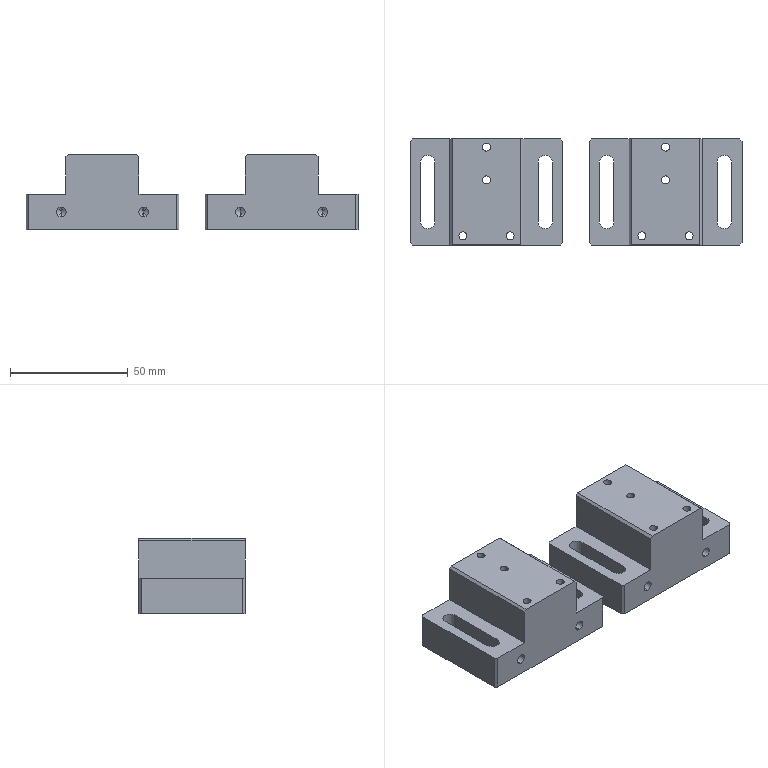NC program | NX | posted with a generic post | part box 140.92 x 45 x 32 mm
Lines 35 to 966 of 10208:
(ZLEVEL_PROFILE_COPY , TOOL : D4)
N68 T11 M6
N70 G54
N72 G17 G0 G90 X8.56 Y15.697 S9500 M3
N74 G43 Z30. H11
N76 Z1.5
N78 G94 G1 Y35.149 Z0.481 F1000.
N80 X8.48 Y35.438 Z0.465
N82 X8.327 Y35.693 Z0.449
N84 X8.057 Y35.936 Z0.43
N86 X7.723 Y36.078 Z0.411
N88 X7.361 Y36.106 Z0.392
N90 X7.009 Y36.014 Z0.373
N92 X6.706 Y35.815 Z0.354
N94 X6.517 Y35.585 Z0.339
N96 X6.415 Y35.375 Z0.326
N98 X6.36 Y35.149 Z0.314
N100 Y22.5 Z-0.349
N102 Y10. F1350.
N104 G3 X7.46 Y8.9 R1.1
N106 X8.56 Y10. R1.1
N108 G1 Y35.
N110 G3 X7.46 Y36.1 R1.1
N112 X6.36 Y35. R1.1
N114 G1 Y22.5
N116 Y11.563 Z-0.416
N118 X6.365 Y10. Z-0.425
N120 X6.381 Y9.817 Z-0.427
N122 X6.405 Y9.717
N124 X6.464 Y9.551 Z-0.428
N126 X6.515 Y9.453 Z-0.429
N128 X6.619 Y9.304 Z-0.43
N130 X6.686 Y9.224 Z-0.431
N132 X6.802 Y9.126 Z-0.432
N134 X6.916 Y9.053 Z-0.433
N136 X7.066 Y8.981 Z-0.434
N138 X7.18 Y8.945
N140 X7.356 Y8.913 Z-0.435
N142 X7.462 Y8.905 Z-0.436
N144 X7.612 Y8.917 Z-0.437
N146 X7.744 Y8.946 Z-0.438
N148 X7.901 Y9. Z-0.439
N150 X8.007 Y9.055 Z-0.44
N152 X8.154 Y9.157 Z-0.441
N154 X8.235 Y9.226
N156 X8.333 Y9.341 Z-0.442
N158 X8.406 Y9.455 Z-0.443
N160 X8.479 Y9.604 Z-0.444
N162 X8.515 Y9.718 Z-0.445
N164 X8.543 Y9.858 Z-0.446
N166 X8.555 Y10. Z-0.447
N168 X8.56 Y11.786 Z-0.458
N170 Y33.214 Z-0.589
N172 X8.555 Y35. Z-0.6
N174 X8.547 Y35.098
N176 X8.535 Y35.196 Z-0.601
N178 X8.511 Y35.297 Z-0.602
N180 X8.482 Y35.385
N182 X8.437 Y35.496 Z-0.603
N184 X8.397 Y35.561 Z-0.604
N186 X8.288 Y35.711 Z-0.605
N188 X8.239 Y35.769
N190 X8.136 Y35.858 Z-0.606
N192 X8.033 Y35.929 Z-0.607
N194 X7.889 Y36.004 Z-0.608
N196 X7.798 Y36.042
N198 X7.669 Y36.073 Z-0.609
N200 X7.542 Y36.089 Z-0.61
N202 X7.381 Y36.09 Z-0.611
N204 X7.281 Y36.08 Z-0.612
N206 X7.145 Y36.048
N208 X7.032 Y36.005 Z-0.613
N210 X6.887 Y35.929 Z-0.614
N212 X6.805 Y35.876 Z-0.615
N214 X6.702 Y35.788 Z-0.616
N216 X6.618 Y35.695
N218 X6.527 Y35.567 Z-0.617
N220 X6.479 Y35.486 Z-0.618
N222 X6.429 Y35.365 Z-0.619
N224 X6.397 Y35.249
N226 X6.375 Y35.125 Z-0.62
N228 X6.365 Y35. Z-0.621
N230 X6.36 Y33.438 Z-0.631
N232 Y22.5 Z-0.698
N234 Y11.563 Z-0.765
N236 X6.365 Y10. Z-0.774
N238 X6.381 Y9.817 Z-0.775
N240 X6.405 Y9.717 Z-0.776
N242 X6.464 Y9.551 Z-0.777
N244 X6.515 Y9.453 Z-0.778
N246 X6.619 Y9.304 Z-0.779
N248 X6.686 Y9.224 Z-0.78
N250 X6.802 Y9.126 Z-0.781
N252 X6.916 Y9.053
N254 X7.066 Y8.981 Z-0.782
N256 X7.18 Y8.945 Z-0.783
N258 X7.356 Y8.913 Z-0.784
N260 X7.462 Y8.905 Z-0.785
N262 X7.612 Y8.917 Z-0.786
N264 X7.744 Y8.946 Z-0.787
N266 X7.901 Y9. Z-0.788
N268 X8.007 Y9.055
N270 X8.154 Y9.157 Z-0.79
N272 X8.235 Y9.226
N274 X8.333 Y9.341 Z-0.791
N276 X8.406 Y9.455 Z-0.792
N278 X8.479 Y9.604 Z-0.793
N280 X8.515 Y9.718 Z-0.794
N282 X8.543 Y9.858 Z-0.795
N284 X8.555 Y10.
N286 X8.56 Y11.786 Z-0.806
N288 Y33.214 Z-0.938
N290 X8.555 Y35. Z-0.949
N292 X8.547 Y35.098
N294 X8.535 Y35.196 Z-0.95
N296 X8.511 Y35.297 Z-0.951
N298 X8.482 Y35.385
N300 X8.437 Y35.496 Z-0.952
N302 X8.397 Y35.561
N304 X8.288 Y35.711 Z-0.954
N306 X8.239 Y35.769
N308 X8.136 Y35.858 Z-0.955
N310 X8.033 Y35.929 Z-0.956
N312 X7.889 Y36.004 Z-0.957
N314 X7.798 Y36.042
N316 X7.669 Y36.073 Z-0.958
N318 X7.542 Y36.089 Z-0.959
N320 X7.381 Y36.09 Z-0.96
N322 X7.281 Y36.08
N324 X7.145 Y36.048 Z-0.961
N326 X7.032 Y36.005 Z-0.962
N328 X6.887 Y35.929 Z-0.963
N330 X6.805 Y35.876 Z-0.964
N332 X6.702 Y35.788
N334 X6.618 Y35.695 Z-0.965
N336 X6.527 Y35.567 Z-0.966
N338 X6.479 Y35.486 Z-0.967
N340 X6.429 Y35.365 Z-0.968
N342 X6.397 Y35.249
N344 X6.375 Y35.125 Z-0.969
N346 X6.365 Y35. Z-0.97
N348 X6.36 Y33.438 Z-0.979
N350 Y22.5 Z-1.047
N352 Y11.563 Z-1.114
N354 X6.365 Y10. Z-1.123
N356 X6.381 Y9.817 Z-1.124
N358 X6.405 Y9.717 Z-1.125
N360 X6.464 Y9.551 Z-1.126
N362 X6.515 Y9.453 Z-1.127
N364 X6.619 Y9.304 Z-1.128
N366 X6.686 Y9.224
N368 X6.802 Y9.126 Z-1.129
N370 X6.916 Y9.053 Z-1.13
N372 X7.066 Y8.981 Z-1.131
N374 X7.18 Y8.945 Z-1.132
N376 X7.356 Y8.913 Z-1.133
N378 X7.462 Y8.905 Z-1.134
N380 X7.612 Y8.917 Z-1.135
N382 X7.744 Y8.946
N384 X7.901 Y9. Z-1.137
N386 X8.007 Y9.055
N388 X8.154 Y9.157 Z-1.138
N390 X8.235 Y9.226 Z-1.139
N392 X8.333 Y9.341 Z-1.14
N394 X8.406 Y9.455 Z-1.141
N396 X8.479 Y9.604 Z-1.142
N398 X8.515 Y9.718 Z-1.143
N400 X8.543 Y9.858
N402 X8.555 Y10. Z-1.144
N404 X8.56 Y11.786 Z-1.155
N406 Y33.214 Z-1.287
N408 X8.555 Y35. Z-1.298
N410 X8.547 Y35.098
N412 X8.535 Y35.196 Z-1.299
N414 X8.511 Y35.297
N416 X8.482 Y35.385 Z-1.3
N418 X8.437 Y35.496 Z-1.301
N420 X8.397 Y35.561
N422 X8.288 Y35.711 Z-1.302
N424 X8.239 Y35.769 Z-1.303
N426 X8.137 Y35.858 Z-1.304
N428 X8.033 Y35.929
N430 X7.889 Y36.004 Z-1.305
N432 X7.798 Y36.042 Z-1.306
N434 X7.669 Y36.073 Z-1.307
N436 X7.542 Y36.089 Z-1.308
N438 X7.381 Y36.09 Z-1.309
N440 X7.281 Y36.08
N442 X7.145 Y36.048 Z-1.31
N444 X7.032 Y36.005 Z-1.311
N446 X6.887 Y35.929 Z-1.312
N448 X6.805 Y35.876
N450 X6.702 Y35.788 Z-1.313
N452 X6.618 Y35.695 Z-1.314
N454 X6.527 Y35.567 Z-1.315
N456 X6.479 Y35.486 Z-1.316
N458 X6.429 Y35.365
N460 X6.397 Y35.249 Z-1.317
N462 X6.375 Y35.125 Z-1.318
N464 X6.365 Y35. Z-1.319
N466 X6.36 Y33.438 Z-1.328
N468 Y22.5 Z-1.395
N470 Y11.563 Z-1.462
N472 X6.365 Y10. Z-1.472
N474 X6.381 Y9.817 Z-1.473
N476 X6.405 Y9.717 Z-1.474
N478 X6.464 Y9.551 Z-1.475
N480 X6.515 Y9.453 Z-1.476
N482 X6.619 Y9.304 Z-1.477
N484 X6.686 Y9.224
N486 X6.802 Y9.126 Z-1.478
N488 X6.916 Y9.053 Z-1.479
N490 X7.066 Y8.981 Z-1.48
N492 X7.18 Y8.945 Z-1.481
N494 X7.356 Y8.913 Z-1.482
N496 X7.462 Y8.905 Z-1.483
N498 X7.612 Y8.917
N500 X7.744 Y8.946 Z-1.484
N502 X7.901 Y9. Z-1.485
N504 X8.007 Y9.055 Z-1.486
N506 X8.154 Y9.157 Z-1.487
N508 X8.235 Y9.226 Z-1.488
N510 X8.333 Y9.341 Z-1.489
N512 X8.406 Y9.455 Z-1.49
N514 X8.479 Y9.604 Z-1.491
N516 X8.515 Y9.718
N518 X8.543 Y9.858 Z-1.492
N520 X8.555 Y10. Z-1.493
N522 X8.56 Y11.786 Z-1.504
N524 Y33.214 Z-1.635
N526 X8.555 Y35. Z-1.646
N528 X8.547 Y35.098 Z-1.647
N530 X8.535 Y35.196 Z-1.648
N532 X8.511 Y35.297
N534 X8.482 Y35.385 Z-1.649
N536 X8.437 Y35.496 Z-1.65
N538 X8.397 Y35.561
N540 X8.288 Y35.711 Z-1.651
N542 X8.239 Y35.769 Z-1.652
N544 X8.137 Y35.858
N546 X8.033 Y35.929 Z-1.653
N548 X7.889 Y36.004 Z-1.654
N550 X7.798 Y36.042 Z-1.655
N552 X7.669 Y36.073 Z-1.656
N554 X7.542 Y36.089
N556 X7.381 Y36.09 Z-1.657
N558 X7.281 Y36.08 Z-1.658
N560 X7.145 Y36.048 Z-1.659
N562 X7.032 Y36.005 Z-1.66
N564 X6.887 Y35.929 Z-1.661
N566 X6.805 Y35.876
N568 X6.702 Y35.788 Z-1.662
N570 X6.618 Y35.695 Z-1.663
N572 X6.527 Y35.567 Z-1.664
N574 X6.479 Y35.486
N576 X6.429 Y35.365 Z-1.665
N578 X6.397 Y35.249 Z-1.666
N580 X6.375 Y35.125 Z-1.667
N582 X6.365 Y35. Z-1.668
N584 X6.36 Y33.438 Z-1.677
N586 Y22.5 Z-1.744
N588 Y11.563 Z-1.811
N590 X6.365 Y10. Z-1.821
N592 X6.381 Y9.817 Z-1.822
N594 X6.405 Y9.717 Z-1.823
N596 X6.464 Y9.551 Z-1.824
N598 X6.515 Y9.453
N600 X6.619 Y9.304 Z-1.825
N602 X6.686 Y9.224 Z-1.826
N604 X6.802 Y9.126 Z-1.827
N606 X6.916 Y9.053 Z-1.828
N608 X7.066 Y8.981 Z-1.829
N610 X7.18 Y8.945 Z-1.83
N612 X7.356 Y8.913 Z-1.831
N614 X7.462 Y8.905
N616 X7.612 Y8.917 Z-1.832
N618 X7.744 Y8.946 Z-1.833
N620 X7.901 Y9. Z-1.834
N622 X8.007 Y9.055 Z-1.835
N624 X8.154 Y9.157 Z-1.836
N626 X8.235 Y9.226 Z-1.837
N628 X8.333 Y9.341 Z-1.838
N630 X8.406 Y9.455
N632 X8.479 Y9.604 Z-1.839
N634 X8.515 Y9.718 Z-1.84
N636 X8.543 Y9.858 Z-1.841
N638 X8.555 Y10. Z-1.842
N640 X8.56 Y11.786 Z-1.853
N642 Y33.214 Z-1.984
N644 X8.555 Y35. Z-1.995
N646 X8.547 Y35.098 Z-1.996
N648 X8.535 Y35.196
N650 X8.511 Y35.297 Z-1.997
N652 X8.482 Y35.385 Z-1.998
N654 X8.437 Y35.496
N656 X8.397 Y35.561 Z-1.999
N658 X8.288 Y35.711 Z-2.
N660 X8.239 Y35.769
N662 X8.137 Y35.858 Z-2.001
N664 X8.033 Y35.929 Z-2.002
N666 X7.889 Y36.004 Z-2.003
N668 X7.798 Y36.042 Z-2.004
N670 X7.669 Y36.073 Z-2.005
N672 X7.542 Y36.089
N674 X7.381 Y36.09 Z-2.006
N676 X7.281 Y36.08 Z-2.007
N678 X7.145 Y36.048 Z-2.008
N680 X7.032 Y36.005 Z-2.009
N682 X6.887 Y35.929 Z-2.01
N684 X6.805 Y35.876
N686 X6.702 Y35.788 Z-2.011
N688 X6.618 Y35.695 Z-2.012
N690 X6.527 Y35.567 Z-2.013
N692 X6.479 Y35.486
N694 X6.429 Y35.365 Z-2.014
N696 X6.397 Y35.249 Z-2.015
N698 X6.375 Y35.125 Z-2.016
N700 X6.365 Y35.
N702 X6.36 Y33.438 Z-2.026
N704 Y22.5 Z-2.093
N706 Y11.563 Z-2.16
N708 X6.365 Y10. Z-2.17
N710 X6.381 Y9.817 Z-2.171
N712 X6.405 Y9.717
N714 X6.464 Y9.551 Z-2.173
N716 X6.515 Y9.453
N718 X6.619 Y9.304 Z-2.174
N720 X6.686 Y9.224 Z-2.175
N722 X6.802 Y9.126 Z-2.176
N724 X6.916 Y9.053 Z-2.177
N726 X7.066 Y8.981 Z-2.178
N728 X7.18 Y8.945
N730 X7.356 Y8.913 Z-2.18
N732 X7.462 Y8.905
N734 X7.612 Y8.917 Z-2.181
N736 X7.744 Y8.946 Z-2.182
N738 X7.901 Y9. Z-2.183
N740 X8.007 Y9.055 Z-2.184
N742 X8.154 Y9.157 Z-2.185
N744 X8.235 Y9.226 Z-2.186
N746 X8.333 Y9.341
N748 X8.406 Y9.455 Z-2.187
N750 X8.479 Y9.604 Z-2.188
N752 X8.515 Y9.718 Z-2.189
N754 X8.543 Y9.858 Z-2.19
N756 X8.555 Y10. Z-2.191
N758 X8.56 Y11.786 Z-2.202
N760 Y33.214 Z-2.333
N762 X8.555 Y35. Z-2.344
N764 X8.547 Y35.098 Z-2.345
N766 X8.535 Y35.196
N768 X8.511 Y35.297 Z-2.346
N770 X8.482 Y35.385 Z-2.347
N772 X8.437 Y35.496
N774 X8.397 Y35.561 Z-2.348
N776 X8.288 Y35.711 Z-2.349
N778 X8.239 Y35.769
N780 X8.137 Y35.858 Z-2.35
N782 X8.033 Y35.929 Z-2.351
N784 X7.889 Y36.004 Z-2.352
N786 X7.798 Y36.042 Z-2.353
N788 X7.669 Y36.073
N790 X7.542 Y36.089 Z-2.354
N792 X7.381 Y36.09 Z-2.355
N794 X7.281 Y36.08 Z-2.356
N796 X7.145 Y36.048 Z-2.357
N798 X7.032 Y36.005
N800 X6.887 Y35.929 Z-2.358
N802 X6.805 Y35.876 Z-2.359
N804 X6.702 Y35.788 Z-2.36
N806 X6.618 Y35.695 Z-2.361
N808 X6.527 Y35.567 Z-2.362
N810 X6.479 Y35.486
N812 X6.429 Y35.365 Z-2.363
N814 X6.397 Y35.249 Z-2.364
N816 X6.375 Y35.125
N818 X6.365 Y35. Z-2.365
N820 X6.36 Y33.438 Z-2.375
N822 Y22.5 Z-2.442
N824 Y11.563 Z-2.509
N826 X6.365 Y10. Z-2.519
N828 X6.381 Y9.817 Z-2.52
N830 X6.405 Y9.717
N832 X6.464 Y9.551 Z-2.521
N834 X6.515 Y9.453 Z-2.522
N836 X6.619 Y9.304 Z-2.523
N838 X6.686 Y9.224 Z-2.524
N840 X6.802 Y9.126 Z-2.525
N842 X6.916 Y9.053 Z-2.526
N844 X7.066 Y8.981 Z-2.527
N846 X7.18 Y8.945
N848 X7.356 Y8.913 Z-2.528
N850 X7.462 Y8.905 Z-2.529
N852 X7.612 Y8.917 Z-2.53
N854 X7.744 Y8.946 Z-2.531
N856 X7.901 Y9. Z-2.532
N858 X8.007 Y9.055 Z-2.533
N860 X8.154 Y9.157 Z-2.534
N862 X8.235 Y9.226
N864 X8.333 Y9.341 Z-2.535
N866 X8.406 Y9.455 Z-2.536
N868 X8.479 Y9.604 Z-2.537
N870 X8.515 Y9.718 Z-2.538
N872 X8.543 Y9.858 Z-2.539
N874 X8.555 Y10. Z-2.54
N876 X8.56 Y11.786 Z-2.551
N878 Y33.214 Z-2.682
N880 X8.555 Y35. Z-2.693
N882 X8.547 Y35.098 Z-2.694
N884 X8.535 Y35.196
N886 X8.511 Y35.297 Z-2.695
N888 X8.482 Y35.385
N890 X8.437 Y35.496 Z-2.696
N892 X8.397 Y35.561 Z-2.697
N894 X8.288 Y35.711 Z-2.698
N896 X8.239 Y35.769
N898 X8.137 Y35.858 Z-2.699
N900 X8.033 Y35.929 Z-2.7
N902 X7.889 Y36.004 Z-2.701
N904 X7.798 Y36.042
N906 X7.669 Y36.073 Z-2.702
N908 X7.542 Y36.089 Z-2.703
N910 X7.381 Y36.09 Z-2.704
N912 X7.281 Y36.08 Z-2.705
N914 X7.145 Y36.048
N916 X7.032 Y36.005 Z-2.706
N918 X6.887 Y35.929 Z-2.707
N920 X6.805 Y35.876 Z-2.708
N922 X6.702 Y35.788 Z-2.709
N924 X6.618 Y35.695
N926 X6.527 Y35.567 Z-2.71
N928 X6.479 Y35.486 Z-2.711
N930 X6.429 Y35.365 Z-2.712
N932 X6.397 Y35.249 Z-2.713
N934 X6.375 Y35.125
N936 X6.365 Y35. Z-2.714
N938 X6.36 Y33.438 Z-2.724
N940 Y22.5 Z-2.791
N942 Y11.563 Z-2.858
N944 X6.365 Y10. Z-2.867
N946 X6.381 Y9.817 Z-2.868
N948 X6.405 Y9.717 Z-2.869
N950 X6.464 Y9.551 Z-2.87
N952 X6.515 Y9.453 Z-2.871
N954 X6.619 Y9.304 Z-2.872
N956 X6.687 Y9.224 Z-2.873
N958 X6.802 Y9.126 Z-2.874
N960 X6.916 Y9.053
N962 X7.066 Y8.981 Z-2.875
N964 X7.18 Y8.945 Z-2.876
N966 X7.356 Y8.913 Z-2.877
N968 X7.462 Y8.905 Z-2.878
N970 X7.612 Y8.917 Z-2.879
N972 X7.744 Y8.946 Z-2.88
N974 X7.901 Y9. Z-2.881
N976 X8.007 Y9.055
N978 X8.154 Y9.157 Z-2.883
N980 X8.235 Y9.226
N982 X8.333 Y9.341 Z-2.884
N984 X8.406 Y9.455 Z-2.885
N986 X8.479 Y9.604 Z-2.886
N988 X8.515 Y9.718 Z-2.887
N990 X8.543 Y9.858 Z-2.888
N992 X8.555 Y10.
N994 X8.56 Y11.786 Z-2.899
N996 Y33.214 Z-3.031
N998 X8.555 Y35. Z-3.042
N1000 X8.547 Y35.098
N1002 X8.535 Y35.196 Z-3.043
N1004 X8.511 Y35.297 Z-3.044
N1006 X8.482 Y35.385
N1008 X8.437 Y35.496 Z-3.045
N1010 X8.397 Y35.561
N1012 X8.288 Y35.711 Z-3.047
N1014 X8.239 Y35.769
N1016 X8.137 Y35.858 Z-3.048
N1018 X8.033 Y35.929 Z-3.049
N1020 X7.889 Y36.004 Z-3.05
N1022 X7.798 Y36.042
N1024 X7.669 Y36.073 Z-3.051
N1026 X7.542 Y36.089 Z-3.052
N1028 X7.381 Y36.09 Z-3.053
N1030 X7.281 Y36.08
N1032 X7.145 Y36.048 Z-3.054
N1034 X7.032 Y36.005 Z-3.055
N1036 X6.887 Y35.929 Z-3.056
N1038 X6.805 Y35.876 Z-3.057
N1040 X6.702 Y35.788
N1042 X6.618 Y35.695 Z-3.058
N1044 X6.527 Y35.567 Z-3.059
N1046 X6.479 Y35.486 Z-3.06
N1048 X6.429 Y35.365 Z-3.061
N1050 X6.397 Y35.249
N1052 X6.375 Y35.125 Z-3.062
N1054 X6.365 Y35. Z-3.063
N1056 X6.36 Y33.438 Z-3.072
N1058 Y22.5 Z-3.14
N1060 Y11.563 Z-3.207
N1062 X6.365 Y10. Z-3.216
N1064 X6.381 Y9.817 Z-3.217
N1066 X6.405 Y9.717 Z-3.218
N1068 X6.464 Y9.551 Z-3.219
N1070 X6.515 Y9.453 Z-3.22
N1072 X6.619 Y9.304 Z-3.221
N1074 X6.687 Y9.224
N1076 X6.802 Y9.126 Z-3.222
N1078 X6.916 Y9.053 Z-3.223
N1080 X7.066 Y8.981 Z-3.224
N1082 X7.18 Y8.945 Z-3.225
N1084 X7.356 Y8.913 Z-3.226
N1086 X7.462 Y8.905 Z-3.227
N1088 X7.612 Y8.917 Z-3.228
N1090 X7.744 Y8.946 Z-3.229
N1092 X7.901 Y9. Z-3.23
N1094 X8.007 Y9.055
N1096 X8.154 Y9.157 Z-3.231
N1098 X8.235 Y9.226 Z-3.232
N1100 X8.333 Y9.341 Z-3.233
N1102 X8.406 Y9.455 Z-3.234
N1104 X8.479 Y9.604 Z-3.235
N1106 X8.515 Y9.718 Z-3.236
N1108 X8.543 Y9.858
N1110 X8.555 Y10. Z-3.237
N1112 X8.56 Y11.786 Z-3.248
N1114 Y33.214 Z-3.38
N1116 X8.555 Y35. Z-3.391
N1118 X8.547 Y35.098
N1120 X8.535 Y35.196 Z-3.392
N1122 X8.511 Y35.297
N1124 X8.482 Y35.385 Z-3.393
N1126 X8.437 Y35.496 Z-3.394
N1128 X8.397 Y35.561
N1130 X8.288 Y35.711 Z-3.395
N1132 X8.239 Y35.769 Z-3.396
N1134 X8.137 Y35.858 Z-3.397
N1136 X8.033 Y35.929
N1138 X7.889 Y36.004 Z-3.398
N1140 X7.798 Y36.042 Z-3.399
N1142 X7.669 Y36.073 Z-3.4
N1144 X7.542 Y36.089 Z-3.401
N1146 X7.381 Y36.09 Z-3.402
N1148 X7.281 Y36.08
N1150 X7.145 Y36.048 Z-3.403
N1152 X7.032 Y36.005 Z-3.404
N1154 X6.887 Y35.929 Z-3.405
N1156 X6.805 Y35.876
N1158 X6.702 Y35.788 Z-3.406
N1160 X6.618 Y35.695 Z-3.407
N1162 X6.527 Y35.567 Z-3.408
N1164 X6.479 Y35.486 Z-3.409
N1166 X6.429 Y35.365
N1168 X6.397 Y35.249 Z-3.41
N1170 X6.375 Y35.125 Z-3.411
N1172 X6.365 Y35. Z-3.412
N1174 X6.36 Y33.438 Z-3.421
N1176 Y22.5 Z-3.488
N1178 Y11.563 Z-3.555
N1180 X6.365 Y10. Z-3.565
N1182 X6.381 Y9.817 Z-3.566
N1184 X6.405 Y9.717 Z-3.567
N1186 X6.464 Y9.551 Z-3.568
N1188 X6.515 Y9.453 Z-3.569
N1190 X6.619 Y9.304 Z-3.57
N1192 X6.687 Y9.224
N1194 X6.802 Y9.126 Z-3.571
N1196 X6.916 Y9.053 Z-3.572
N1198 X7.066 Y8.981 Z-3.573
N1200 X7.18 Y8.945 Z-3.574
N1202 X7.356 Y8.913 Z-3.575
N1204 X7.462 Y8.905 Z-3.576
N1206 X7.612 Y8.917 Z-3.577
N1208 X7.744 Y8.946
N1210 X7.901 Y9. Z-3.578
N1212 X8.007 Y9.055 Z-3.579
N1214 X8.154 Y9.157 Z-3.58
N1216 X8.235 Y9.226 Z-3.581
N1218 X8.333 Y9.341 Z-3.582
N1220 X8.406 Y9.455 Z-3.583
N1222 X8.479 Y9.604 Z-3.584
N1224 X8.515 Y9.718
N1226 X8.543 Y9.858 Z-3.585
N1228 X8.555 Y10. Z-3.586
N1230 X8.56 Y11.786 Z-3.597
N1232 Y33.214 Z-3.728
N1234 X8.555 Y35. Z-3.739
N1236 X8.547 Y35.098 Z-3.74
N1238 X8.535 Y35.196 Z-3.741
N1240 X8.511 Y35.297
N1242 X8.482 Y35.385 Z-3.742
N1244 X8.437 Y35.496 Z-3.743
N1246 X8.397 Y35.561
N1248 X8.288 Y35.711 Z-3.744
N1250 X8.239 Y35.769 Z-3.745
N1252 X8.137 Y35.858 Z-3.746
N1254 X8.033 Y35.929
N1256 X7.889 Y36.004 Z-3.747
N1258 X7.798 Y36.042 Z-3.748
N1260 X7.669 Y36.073 Z-3.749
N1262 X7.542 Y36.089
N1264 X7.381 Y36.09 Z-3.75
N1266 X7.281 Y36.08 Z-3.751
N1268 X7.145 Y36.048 Z-3.752
N1270 X7.032 Y36.005 Z-3.753
N1272 X6.887 Y35.929 Z-3.754
N1274 X6.805 Y35.876
N1276 X6.702 Y35.788 Z-3.755
N1278 X6.618 Y35.695 Z-3.756
N1280 X6.527 Y35.567 Z-3.757
N1282 X6.479 Y35.486
N1284 X6.429 Y35.365 Z-3.758
N1286 X6.397 Y35.249 Z-3.759
N1288 X6.375 Y35.125 Z-3.76
N1290 X6.365 Y35. Z-3.761
N1292 X6.36 Y33.438 Z-3.77
N1294 Y22.5 Z-3.837
N1296 Y11.563 Z-3.904
N1298 X6.365 Y10. Z-3.914
N1300 X6.381 Y9.817 Z-3.915
N1302 X6.405 Y9.717 Z-3.916
N1304 X6.464 Y9.551 Z-3.917
N1306 X6.515 Y9.453
N1308 X6.619 Y9.304 Z-3.918
N1310 X6.687 Y9.224 Z-3.919
N1312 X6.802 Y9.126 Z-3.92
N1314 X6.916 Y9.053 Z-3.921
N1316 X7.066 Y8.981 Z-3.922
N1318 X7.18 Y8.945 Z-3.923
N1320 X7.356 Y8.913 Z-3.924
N1322 X7.462 Y8.905
N1324 X7.612 Y8.917 Z-3.925
N1326 X7.744 Y8.946 Z-3.926
N1328 X7.901 Y9.001 Z-3.927
N1330 X8.007 Y9.055 Z-3.928
N1332 X8.154 Y9.157 Z-3.929
N1334 X8.235 Y9.226 Z-3.93
N1336 X8.333 Y9.341 Z-3.931
N1338 X8.406 Y9.455
N1340 X8.478 Y9.604 Z-3.932
N1342 X8.515 Y9.718 Z-3.933
N1344 X8.545 Y9.858 Z-3.934
N1346 X8.555 Y10. Z-3.935
N1348 X8.56 Y11.786 Z-3.946
N1350 Y33.214 Z-4.077
N1352 X8.555 Y35. Z-4.088
N1354 X8.547 Y35.098 Z-4.089
N1356 X8.535 Y35.196
N1358 X8.511 Y35.297 Z-4.09
N1360 X8.482 Y35.385 Z-4.091
N1362 X8.437 Y35.496
N1364 X8.397 Y35.561 Z-4.092
N1366 X8.288 Y35.711 Z-4.093
N1368 X8.239 Y35.769 Z-4.094
N1370 X8.137 Y35.858
N1372 X8.033 Y35.929 Z-4.095
N1374 X7.889 Y36.004 Z-4.096
N1376 X7.798 Y36.042 Z-4.097
N1378 X7.669 Y36.073 Z-4.098
N1380 X7.542 Y36.089
N1382 X7.381 Y36.09 Z-4.099
N1384 X7.281 Y36.08 Z-4.1
N1386 X7.145 Y36.048 Z-4.101
N1388 X7.032 Y36.005 Z-4.102
N1390 X6.887 Y35.929 Z-4.103
N1392 X6.805 Y35.876
N1394 X6.702 Y35.788 Z-4.104
N1396 X6.618 Y35.695 Z-4.105
N1398 X6.527 Y35.567 Z-4.106
N1400 X6.479 Y35.486
N1402 X6.429 Y35.365 Z-4.107
N1404 X6.397 Y35.249 Z-4.108
N1406 X6.375 Y35.125 Z-4.109
N1408 X6.365 Y35.
N1410 X6.36 Y33.438 Z-4.119
N1412 Y22.5 Z-4.186
N1414 Y11.563 Z-4.253
N1416 X6.365 Y10. Z-4.263
N1418 X6.381 Y9.817 Z-4.264
N1420 X6.405 Y9.717
N1422 X6.464 Y9.551 Z-4.266
N1424 X6.515 Y9.453
N1426 X6.619 Y9.304 Z-4.267
N1428 X6.687 Y9.224 Z-4.268
N1430 X6.802 Y9.126 Z-4.269
N1432 X6.916 Y9.053 Z-4.27
N1434 X7.066 Y8.981 Z-4.271
N1436 X7.18 Y8.945 Z-4.272
N1438 X7.356 Y8.913 Z-4.273
N1440 X7.462 Y8.905
N1442 X7.612 Y8.917 Z-4.274
N1444 X7.744 Y8.946 Z-4.275
N1446 X7.901 Y9.001 Z-4.276
N1448 X8.007 Y9.055 Z-4.277
N1450 X8.154 Y9.157 Z-4.278
N1452 X8.235 Y9.226 Z-4.279
N1454 X8.333 Y9.341
N1456 X8.406 Y9.455 Z-4.28
N1458 X8.478 Y9.604 Z-4.281
N1460 X8.515 Y9.718 Z-4.282
N1462 X8.545 Y9.858 Z-4.283
N1464 X8.555 Y10. Z-4.284
N1466 X8.56 Y11.786 Z-4.295
N1468 Y33.214 Z-4.426
N1470 X8.555 Y35. Z-4.437
N1472 X8.547 Y35.098 Z-4.438
N1474 X8.535 Y35.196
N1476 X8.511 Y35.297 Z-4.439
N1478 X8.482 Y35.385 Z-4.44
N1480 X8.437 Y35.496
N1482 X8.397 Y35.561 Z-4.441
N1484 X8.289 Y35.712 Z-4.442
N1486 X8.239 Y35.769
N1488 X8.133 Y35.861 Z-4.443
N1490 X8.033 Y35.929 Z-4.444
N1492 X7.888 Y36.005 Z-4.445
N1494 X7.798 Y36.042 Z-4.446
N1496 X7.669 Y36.073
N1498 X7.542 Y36.089 Z-4.447
N1500 X7.381 Y36.09 Z-4.448
N1502 X7.281 Y36.08 Z-4.449
N1504 X7.145 Y36.048 Z-4.45
N1506 X7.032 Y36.005
N1508 X6.887 Y35.929 Z-4.451
N1510 X6.805 Y35.876 Z-4.452
N1512 X6.702 Y35.788 Z-4.453
N1514 X6.618 Y35.695 Z-4.454
N1516 X6.527 Y35.567 Z-4.455
N1518 X6.479 Y35.486
N1520 X6.429 Y35.365 Z-4.456
N1522 X6.397 Y35.249 Z-4.457
N1524 X6.375 Y35.125
N1526 X6.365 Y35. Z-4.458
N1528 X6.36 Y33.438 Z-4.468
N1530 Y22.5 Z-4.535
N1532 Y11.563 Z-4.602
N1534 X6.365 Y10. Z-4.612
N1536 X6.381 Y9.817 Z-4.613
N1538 X6.405 Y9.717
N1540 X6.464 Y9.551 Z-4.614
N1542 X6.515 Y9.453 Z-4.615
N1544 X6.619 Y9.304 Z-4.616
N1546 X6.687 Y9.224 Z-4.617
N1548 X6.802 Y9.126 Z-4.618
N1550 X6.916 Y9.053 Z-4.619
N1552 X7.066 Y8.981 Z-4.62
N1554 X7.18 Y8.945
N1556 X7.356 Y8.913 Z-4.621
N1558 X7.462 Y8.905 Z-4.622
N1560 X7.612 Y8.917 Z-4.623
N1562 X7.744 Y8.946 Z-4.624
N1564 X7.901 Y9.001 Z-4.625
N1566 X8.007 Y9.055 Z-4.626
N1568 X8.154 Y9.157 Z-4.627
N1570 X8.235 Y9.226
N1572 X8.333 Y9.341 Z-4.628
N1574 X8.406 Y9.455 Z-4.629
N1576 X8.478 Y9.604 Z-4.63
N1578 X8.515 Y9.718 Z-4.631
N1580 X8.545 Y9.858 Z-4.632
N1582 X8.555 Y10. Z-4.633
N1584 X8.56 Y11.786 Z-4.644
N1586 Y33.214 Z-4.775
N1588 X8.555 Y35. Z-4.786
N1590 X8.547 Y35.098 Z-4.787
N1592 X8.535 Y35.196
N1594 X8.511 Y35.297 Z-4.788
N1596 X8.482 Y35.385
N1598 X8.437 Y35.495 Z-4.789
N1600 X8.397 Y35.561 Z-4.79
N1602 X8.289 Y35.712 Z-4.791
N1604 X8.239 Y35.769
N1606 X8.133 Y35.861 Z-4.792
N1608 X8.033 Y35.929 Z-4.793
N1610 X7.888 Y36.005 Z-4.794
N1612 X7.798 Y36.042
N1614 X7.669 Y36.073 Z-4.795
N1616 X7.542 Y36.089 Z-4.796
N1618 X7.381 Y36.09 Z-4.797
N1620 X7.281 Y36.08 Z-4.798
N1622 X7.145 Y36.048
N1624 X7.032 Y36.005 Z-4.799
N1626 X6.887 Y35.929 Z-4.8
N1628 X6.805 Y35.876 Z-4.801
N1630 X6.702 Y35.788 Z-4.802
N1632 X6.618 Y35.695
N1634 X6.527 Y35.567 Z-4.803
N1636 X6.479 Y35.486 Z-4.804
N1638 X6.429 Y35.365 Z-4.805
N1640 X6.397 Y35.249 Z-4.806
N1642 X6.375 Y35.125
N1644 X6.365 Y35. Z-4.807
N1646 X6.36 Y33.438 Z-4.817
N1648 Y22.5 Z-4.884
N1650 Y11.563 Z-4.951
N1652 X6.365 Y10. Z-4.96
N1654 X6.381 Y9.817 Z-4.961
N1656 X6.405 Y9.717 Z-4.962
N1658 X6.464 Y9.551 Z-4.963
N1660 X6.515 Y9.453 Z-4.964
N1662 X6.619 Y9.304 Z-4.965
N1664 X6.687 Y9.224 Z-4.966
N1666 X6.802 Y9.126 Z-4.967
N1668 X6.916 Y9.053
N1670 X7.066 Y8.981 Z-4.968
N1672 X7.18 Y8.945 Z-4.969
N1674 X7.356 Y8.913 Z-4.97
N1676 X7.462 Y8.905 Z-4.971
N1678 X7.612 Y8.917 Z-4.972
N1680 X7.744 Y8.946 Z-4.973
N1682 X7.901 Y9.001 Z-4.974
N1684 X8.007 Y9.055
N1686 X8.154 Y9.157 Z-4.976
N1688 X8.235 Y9.226
N1690 X8.333 Y9.341 Z-4.977
N1692 X8.406 Y9.455 Z-4.978
N1694 X8.478 Y9.604 Z-4.979
N1696 X8.515 Y9.718 Z-4.98
N1698 X8.545 Y9.858 Z-4.981
N1700 X8.555 Y10.
N1702 X8.56 Y11.786 Z-4.992
N1704 Y33.214 Z-5.124
N1706 X8.555 Y35. Z-5.135
N1708 X8.547 Y35.098
N1710 X8.535 Y35.196 Z-5.136
N1712 X8.511 Y35.297 Z-5.137
N1714 X8.482 Y35.385
N1716 X8.437 Y35.495 Z-5.138
N1718 X8.397 Y35.561
N1720 X8.289 Y35.712 Z-5.14
N1722 X8.239 Y35.769
N1724 X8.133 Y35.861 Z-5.141
N1726 X8.033 Y35.929 Z-5.142
N1728 X7.888 Y36.005 Z-5.143
N1730 X7.798 Y36.042
N1732 X7.669 Y36.073 Z-5.144
N1734 X7.542 Y36.089 Z-5.145
N1736 X7.381 Z-5.146
N1738 X7.281 Y36.08
N1740 X7.145 Y36.048 Z-5.147
N1742 X7.032 Y36.005 Z-5.148
N1744 X6.887 Y35.929 Z-5.149
N1746 X6.805 Y35.876 Z-5.15
N1748 X6.702 Y35.788 Z-5.151
N1750 X6.618 Y35.695
N1752 X6.527 Y35.567 Z-5.152
N1754 X6.479 Y35.486 Z-5.153
N1756 X6.429 Y35.365 Z-5.154
N1758 X6.397 Y35.249
N1760 X6.375 Y35.125 Z-5.155
N1762 X6.365 Y35. Z-5.156
N1764 X6.36 Y33.438 Z-5.165
N1766 Y22.5 Z-5.233
N1768 Y11.563 Z-5.3
N1770 X6.365 Y10. Z-5.309
N1772 X6.381 Y9.817 Z-5.31
N1774 X6.405 Y9.717 Z-5.311
N1776 X6.464 Y9.551 Z-5.312
N1778 X6.515 Y9.453 Z-5.313
N1780 X6.619 Y9.304 Z-5.314
N1782 X6.687 Y9.224
N1784 X6.802 Y9.126 Z-5.315
N1786 X6.916 Y9.053 Z-5.316
N1788 X7.066 Y8.981 Z-5.317
N1790 X7.18 Y8.945 Z-5.318
N1792 X7.356 Y8.913 Z-5.319
N1794 X7.462 Y8.905 Z-5.32
N1796 X7.612 Y8.917 Z-5.321
N1798 X7.744 Y8.946 Z-5.322
N1800 X7.901 Y9.001 Z-5.323
N1802 X8.007 Y9.055
N1804 X8.154 Y9.157 Z-5.324
N1806 X8.235 Y9.226 Z-5.325
N1808 X8.333 Y9.341 Z-5.326
N1810 X8.406 Y9.455 Z-5.327
N1812 X8.478 Y9.604 Z-5.328
N1814 X8.515 Y9.718 Z-5.329
N1816 X8.545 Y9.858
N1818 X8.555 Y10. Z-5.33
N1820 X8.56 Y11.786 Z-5.341
N1822 Y33.214 Z-5.473
N1824 X8.555 Y35. Z-5.484
N1826 X8.547 Y35.098
N1828 X8.535 Y35.196 Z-5.485
N1830 X8.511 Y35.297
N1832 X8.482 Y35.385 Z-5.486
N1834 X8.437 Y35.495 Z-5.487
N1836 X8.397 Y35.561
N1838 X8.289 Y35.712 Z-5.488
N1840 X8.239 Y35.769 Z-5.489
N1842 X8.133 Y35.861 Z-5.49
N1844 X8.033 Y35.929
N1846 X7.888 Y36.005 Z-5.491
N1848 X7.798 Y36.042 Z-5.492
N1850 X7.669 Y36.073 Z-5.493
N1852 X7.542 Y36.089 Z-5.494
N1854 X7.381 Z-5.495
N1856 X7.281 Y36.08
N1858 X7.145 Y36.048 Z-5.496
N1860 X7.032 Y36.005 Z-5.497
N1862 X6.887 Y35.929 Z-5.498
N1864 X6.805 Y35.876 Z-5.499
N1866 X6.702 Y35.788
N1868 X6.618 Y35.695 Z-5.5
N1870 X6.527 Y35.567 Z-5.501
N1872 X6.479 Y35.486 Z-5.502
N1874 X6.429 Y35.365
N1876 X6.397 Y35.249 Z-5.503
N1878 X6.375 Y35.125 Z-5.504
N1880 X6.365 Y35. Z-5.505
N1882 X6.36 Y33.438 Z-5.514
N1884 Y22.5 Z-5.581
N1886 Y11.563 Z-5.648
N1888 X6.365 Y10. Z-5.658
N1890 X6.381 Y9.817 Z-5.659
N1892 X6.405 Y9.717 Z-5.66
N1894 X6.464 Y9.551 Z-5.661
N1896 X6.515 Y9.453 Z-5.662
N1898 X6.619 Y9.304 Z-5.663
N1900 X6.687 Y9.224
N1902 X6.802 Y9.126 Z-5.664
N1904 X6.916 Y9.053 Z-5.665
N1906 X7.066 Y8.981 Z-5.666
N1908 X7.18 Y8.945 Z-5.667
N1910 X7.356 Y8.913 Z-5.668
N1912 X7.462 Y8.905 Z-5.669
N1914 X7.612 Y8.917 Z-5.67
N1916 X7.744 Y8.946
N1918 X7.901 Y9.001 Z-5.671
N1920 X8.007 Y9.055 Z-5.672
N1922 X8.154 Y9.157 Z-5.673
N1924 X8.235 Y9.226 Z-5.674